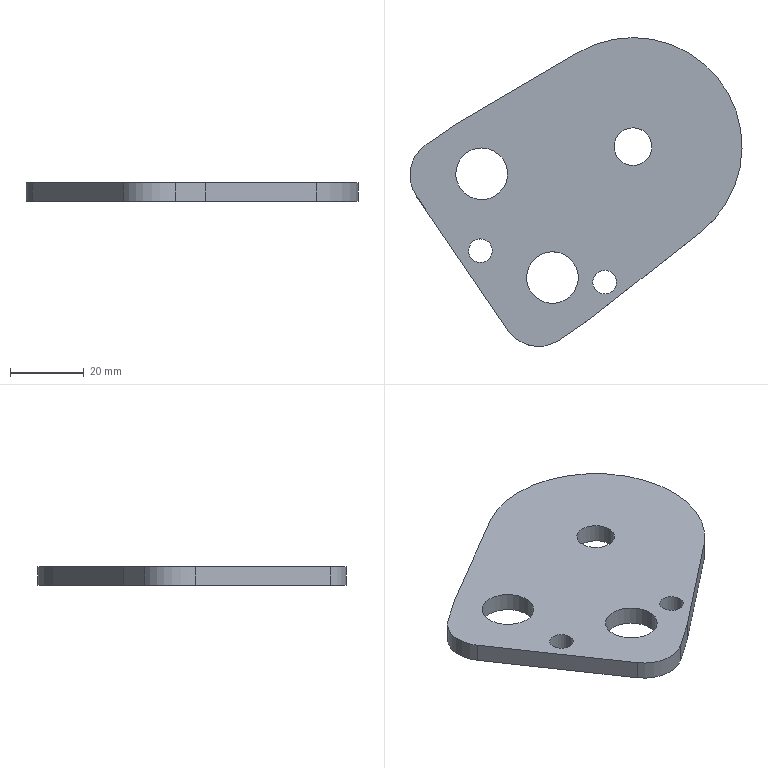Part | NX | features solid 2 | 1 solid | 15 faces | box 89.902 x 83.584 x 5 mm | volume 21833 mm3 | cylinder 8 | plane 7 | commonest cylinder face diameters 6.4 x2 14 x2 20 x2 10.2 x1 59 x1
STEP:
#1=CARTESIAN_POINT('',(-192.435,38.031,115.));
#2=VERTEX_POINT('',#1);
#3=CARTESIAN_POINT('',(-159.285,-10.613,115.));
#4=VERTEX_POINT('',#3);
#5=CARTESIAN_POINT('',(-177.504,12.589,115.));
#6=DIRECTION('',(0.,0.,-1.));
#7=DIRECTION('',(-0.8264,-0.5631,0.));
#8=AXIS2_PLACEMENT_3D('',#5,#6,#7);
#9=CIRCLE('',#8,29.5);
#10=EDGE_CURVE('',#2,#4,#9,.T.);
#11=ORIENTED_EDGE('',*,*,#10,.F.);
#12=CARTESIAN_POINT('',(-192.435,38.031,120.));
#13=VERTEX_POINT('',#12);
#14=CARTESIAN_POINT('',(-192.435,38.031,120.));
#15=DIRECTION('',(0.,0.,-1.));
#16=VECTOR('',#15,1000.);
#17=LINE('',#14,#16);
#18=EDGE_CURVE('',#13,#2,#17,.T.);
#19=ORIENTED_EDGE('',*,*,#18,.F.);
#20=CARTESIAN_POINT('',(-159.285,-10.613,120.));
#21=VERTEX_POINT('',#20);
#22=CARTESIAN_POINT('',(-177.504,12.589,120.));
#23=DIRECTION('',(0.,0.,-1.));
#24=DIRECTION('',(-0.8264,-0.5631,0.));
#25=AXIS2_PLACEMENT_3D('',#22,#23,#24);
#26=CIRCLE('',#25,29.5);
#27=EDGE_CURVE('',#13,#21,#26,.T.);
#28=ORIENTED_EDGE('',*,*,#27,.T.);
#29=CARTESIAN_POINT('',(-159.285,-10.613,120.));
#30=DIRECTION('',(0.,0.,-1.));
#31=VECTOR('',#30,1000.);
#32=LINE('',#29,#31);
#33=EDGE_CURVE('',#21,#4,#32,.T.);
#34=ORIENTED_EDGE('',*,*,#33,.T.);
#35=EDGE_LOOP('',(#11,#19,#28,#34));
#36=FACE_BOUND('',#35,.T.);
#37=CARTESIAN_POINT('',(-177.504,12.589,120.));
#38=DIRECTION('',(0.,0.,-1.));
#39=DIRECTION('',(-0.8264,-0.5631,0.));
#40=AXIS2_PLACEMENT_3D('',#37,#38,#39);
#41=CYLINDRICAL_SURFACE('',#40,29.5);
#42=ADVANCED_FACE('',(#36),#41,.T.);
#43=CARTESIAN_POINT('',(-189.232,-34.128,115.));
#44=VERTEX_POINT('',#43);
#45=CARTESIAN_POINT('',(-189.232,-34.128,115.));
#46=DIRECTION('',(0.7865,0.6176,0.));
#47=VECTOR('',#46,1000.);
#48=LINE('',#45,#47);
#49=EDGE_CURVE('',#44,#4,#48,.T.);
#50=ORIENTED_EDGE('',*,*,#49,.T.);
#51=ORIENTED_EDGE('',*,*,#33,.F.);
#52=CARTESIAN_POINT('',(-189.232,-34.128,120.));
#53=VERTEX_POINT('',#52);
#54=CARTESIAN_POINT('',(-189.232,-34.128,120.));
#55=DIRECTION('',(0.7865,0.6176,0.));
#56=VECTOR('',#55,1000.);
#57=LINE('',#54,#56);
#58=EDGE_CURVE('',#53,#21,#57,.T.);
#59=ORIENTED_EDGE('',*,*,#58,.F.);
#60=CARTESIAN_POINT('',(-189.232,-34.128,120.));
#61=DIRECTION('',(0.,0.,-1.));
#62=VECTOR('',#61,1000.);
#63=LINE('',#60,#62);
#64=EDGE_CURVE('',#53,#44,#63,.T.);
#65=ORIENTED_EDGE('',*,*,#64,.T.);
#66=EDGE_LOOP('',(#50,#51,#59,#65));
#67=FACE_BOUND('',#66,.T.);
#68=CARTESIAN_POINT('',(-189.232,-34.128,120.));
#69=DIRECTION('',(-0.6176,0.7865,0.));
#70=DIRECTION('',(0.7865,0.6176,0.));
#71=AXIS2_PLACEMENT_3D('',#68,#69,#70);
#72=PLANE('',#71);
#73=ADVANCED_FACE('',(#67),#72,.F.);
#74=CARTESIAN_POINT('',(-197.496,-39.759,120.));
#75=VERTEX_POINT('',#74);
#76=CARTESIAN_POINT('',(-189.232,-34.128,120.));
#77=DIRECTION('',(-0.8264,-0.5631,0.));
#78=VECTOR('',#77,1000.);
#79=LINE('',#76,#78);
#80=EDGE_CURVE('',#53,#75,#79,.T.);
#81=ORIENTED_EDGE('',*,*,#80,.T.);
#82=CARTESIAN_POINT('',(-197.496,-39.759,115.));
#83=VERTEX_POINT('',#82);
#84=CARTESIAN_POINT('',(-197.496,-39.759,120.));
#85=DIRECTION('',(0.,0.,-1.));
#86=VECTOR('',#85,1000.);
#87=LINE('',#84,#86);
#88=EDGE_CURVE('',#75,#83,#87,.T.);
#89=ORIENTED_EDGE('',*,*,#88,.T.);
#90=CARTESIAN_POINT('',(-189.232,-34.128,115.));
#91=DIRECTION('',(-0.8264,-0.5631,0.));
#92=VECTOR('',#91,1000.);
#93=LINE('',#90,#92);
#94=EDGE_CURVE('',#44,#83,#93,.T.);
#95=ORIENTED_EDGE('',*,*,#94,.F.);
#96=ORIENTED_EDGE('',*,*,#64,.F.);
#97=EDGE_LOOP('',(#81,#89,#95,#96));
#98=FACE_BOUND('',#97,.T.);
#99=CARTESIAN_POINT('',(-189.232,-34.128,120.));
#100=DIRECTION('',(0.5631,-0.8264,0.));
#101=DIRECTION('',(0.,0.,1.));
#102=AXIS2_PLACEMENT_3D('',#99,#100,#101);
#103=PLANE('',#102);
#104=ADVANCED_FACE('',(#98),#103,.T.);
#105=CARTESIAN_POINT('',(-211.391,-37.127,120.));
#106=VERTEX_POINT('',#105);
#107=CARTESIAN_POINT('',(-236.169,-0.7668,120.));
#108=VERTEX_POINT('',#107);
#109=CARTESIAN_POINT('',(-205.76,-45.39,120.));
#110=DIRECTION('',(-0.5631,0.8264,0.));
#111=VECTOR('',#110,1000.);
#112=LINE('',#109,#111);
#113=EDGE_CURVE('',#106,#108,#112,.T.);
#114=ORIENTED_EDGE('',*,*,#113,.T.);
#115=CARTESIAN_POINT('',(-236.169,-0.7668,115.));
#116=VERTEX_POINT('',#115);
#117=CARTESIAN_POINT('',(-236.169,-0.7668,120.));
#118=DIRECTION('',(0.,0.,-1.));
#119=VECTOR('',#118,1000.);
#120=LINE('',#117,#119);
#121=EDGE_CURVE('',#108,#116,#120,.T.);
#122=ORIENTED_EDGE('',*,*,#121,.T.);
#123=CARTESIAN_POINT('',(-211.391,-37.127,115.));
#124=VERTEX_POINT('',#123);
#125=CARTESIAN_POINT('',(-205.76,-45.39,115.));
#126=DIRECTION('',(-0.5631,0.8264,0.));
#127=VECTOR('',#126,1000.);
#128=LINE('',#125,#127);
#129=EDGE_CURVE('',#124,#116,#128,.T.);
#130=ORIENTED_EDGE('',*,*,#129,.F.);
#131=CARTESIAN_POINT('',(-211.391,-37.127,120.));
#132=DIRECTION('',(0.,0.,-1.));
#133=VECTOR('',#132,1000.);
#134=LINE('',#131,#133);
#135=EDGE_CURVE('',#124,#106,#134,.F.);
#136=ORIENTED_EDGE('',*,*,#135,.T.);
#137=EDGE_LOOP('',(#114,#122,#130,#136));
#138=FACE_BOUND('',#137,.T.);
#139=CARTESIAN_POINT('',(-205.76,-45.39,120.));
#140=DIRECTION('',(-0.8264,-0.5631,0.));
#141=DIRECTION('',(0.,0.,1.));
#142=AXIS2_PLACEMENT_3D('',#139,#140,#141);
#143=PLANE('',#142);
#144=ADVANCED_FACE('',(#138),#143,.T.);
#145=CARTESIAN_POINT('',(-233.537,13.128,115.));
#146=VERTEX_POINT('',#145);
#147=CARTESIAN_POINT('',(-225.273,18.76,115.));
#148=VERTEX_POINT('',#147);
#149=CARTESIAN_POINT('',(-241.8,7.497,115.));
#150=DIRECTION('',(0.8264,0.5631,0.));
#151=VECTOR('',#150,1000.);
#152=LINE('',#149,#151);
#153=EDGE_CURVE('',#146,#148,#152,.T.);
#154=ORIENTED_EDGE('',*,*,#153,.F.);
#155=CARTESIAN_POINT('',(-233.537,13.128,120.));
#156=VERTEX_POINT('',#155);
#157=CARTESIAN_POINT('',(-233.537,13.128,120.));
#158=DIRECTION('',(0.,0.,-1.));
#159=VECTOR('',#158,1000.);
#160=LINE('',#157,#159);
#161=EDGE_CURVE('',#146,#156,#160,.F.);
#162=ORIENTED_EDGE('',*,*,#161,.T.);
#163=CARTESIAN_POINT('',(-225.273,18.76,120.));
#164=VERTEX_POINT('',#163);
#165=CARTESIAN_POINT('',(-241.8,7.497,120.));
#166=DIRECTION('',(0.8264,0.5631,0.));
#167=VECTOR('',#166,1000.);
#168=LINE('',#165,#167);
#169=EDGE_CURVE('',#156,#164,#168,.T.);
#170=ORIENTED_EDGE('',*,*,#169,.T.);
#171=CARTESIAN_POINT('',(-225.273,18.76,120.));
#172=DIRECTION('',(0.,0.,-1.));
#173=VECTOR('',#172,1000.);
#174=LINE('',#171,#173);
#175=EDGE_CURVE('',#164,#148,#174,.T.);
#176=ORIENTED_EDGE('',*,*,#175,.T.);
#177=EDGE_LOOP('',(#154,#162,#170,#176));
#178=FACE_BOUND('',#177,.T.);
#179=CARTESIAN_POINT('',(-241.8,7.497,120.));
#180=DIRECTION('',(-0.5631,0.8264,0.));
#181=DIRECTION('',(0.,0.,-1.));
#182=AXIS2_PLACEMENT_3D('',#179,#180,#181);
#183=PLANE('',#182);
#184=ADVANCED_FACE('',(#178),#183,.T.);
#185=CARTESIAN_POINT('',(-181.718,9.717,120.));
#186=VERTEX_POINT('',#185);
#187=CARTESIAN_POINT('',(-177.504,12.589,120.));
#188=DIRECTION('',(0.,0.,-1.));
#189=DIRECTION('',(-0.8264,-0.5631,0.));
#190=AXIS2_PLACEMENT_3D('',#187,#188,#189);
#191=CIRCLE('',#190,5.1);
#192=EDGE_CURVE('',#186,#186,#191,.T.);
#193=ORIENTED_EDGE('',*,*,#192,.F.);
#194=EDGE_LOOP('',(#193));
#195=FACE_BOUND('',#194,.T.);
#196=CARTESIAN_POINT('',(-181.718,9.717,115.));
#197=VERTEX_POINT('',#196);
#198=CARTESIAN_POINT('',(-177.504,12.589,115.));
#199=DIRECTION('',(0.,0.,-1.));
#200=DIRECTION('',(-0.8264,-0.5631,0.));
#201=AXIS2_PLACEMENT_3D('',#198,#199,#200);
#202=CIRCLE('',#201,5.1);
#203=EDGE_CURVE('',#197,#197,#202,.T.);
#204=ORIENTED_EDGE('',*,*,#203,.T.);
#205=EDGE_LOOP('',(#204));
#206=FACE_BOUND('',#205,.T.);
#207=CARTESIAN_POINT('',(-177.504,12.589,120.));
#208=DIRECTION('',(0.,0.,-1.));
#209=DIRECTION('',(-0.8264,-0.5631,0.));
#210=AXIS2_PLACEMENT_3D('',#207,#208,#209);
#211=CYLINDRICAL_SURFACE('',#210,5.1);
#212=ADVANCED_FACE('',(#195,#206),#211,.F.);
#213=CARTESIAN_POINT('',(-205.117,-26.8,120.));
#214=VERTEX_POINT('',#213);
#215=CARTESIAN_POINT('',(-199.332,-22.858,120.));
#216=DIRECTION('',(0.,0.,-1.));
#217=DIRECTION('',(-0.8264,-0.5631,0.));
#218=AXIS2_PLACEMENT_3D('',#215,#216,#217);
#219=CIRCLE('',#218,7.);
#220=EDGE_CURVE('',#214,#214,#219,.T.);
#221=ORIENTED_EDGE('',*,*,#220,.F.);
#222=EDGE_LOOP('',(#221));
#223=FACE_BOUND('',#222,.T.);
#224=CARTESIAN_POINT('',(-205.117,-26.8,115.));
#225=VERTEX_POINT('',#224);
#226=CARTESIAN_POINT('',(-199.332,-22.858,115.));
#227=DIRECTION('',(0.,0.,-1.));
#228=DIRECTION('',(-0.8264,-0.5631,0.));
#229=AXIS2_PLACEMENT_3D('',#226,#227,#228);
#230=CIRCLE('',#229,7.);
#231=EDGE_CURVE('',#225,#225,#230,.T.);
#232=ORIENTED_EDGE('',*,*,#231,.T.);
#233=EDGE_LOOP('',(#232));
#234=FACE_BOUND('',#233,.T.);
#235=CARTESIAN_POINT('',(-199.332,-22.858,120.));
#236=DIRECTION('',(0.,0.,-1.));
#237=DIRECTION('',(-0.8264,-0.5631,0.));
#238=AXIS2_PLACEMENT_3D('',#235,#236,#237);
#239=CYLINDRICAL_SURFACE('',#238,7.);
#240=ADVANCED_FACE('',(#223,#234),#239,.F.);
#241=CARTESIAN_POINT('',(-224.263,1.296,120.));
#242=VERTEX_POINT('',#241);
#243=CARTESIAN_POINT('',(-218.479,5.238,120.));
#244=DIRECTION('',(0.,0.,-1.));
#245=DIRECTION('',(-0.8264,-0.5631,0.));
#246=AXIS2_PLACEMENT_3D('',#243,#244,#245);
#247=CIRCLE('',#246,7.);
#248=EDGE_CURVE('',#242,#242,#247,.T.);
#249=ORIENTED_EDGE('',*,*,#248,.F.);
#250=EDGE_LOOP('',(#249));
#251=FACE_BOUND('',#250,.T.);
#252=CARTESIAN_POINT('',(-224.263,1.296,115.));
#253=VERTEX_POINT('',#252);
#254=CARTESIAN_POINT('',(-218.479,5.238,115.));
#255=DIRECTION('',(0.,0.,-1.));
#256=DIRECTION('',(-0.8264,-0.5631,0.));
#257=AXIS2_PLACEMENT_3D('',#254,#255,#256);
#258=CIRCLE('',#257,7.);
#259=EDGE_CURVE('',#253,#253,#258,.T.);
#260=ORIENTED_EDGE('',*,*,#259,.T.);
#261=EDGE_LOOP('',(#260));
#262=FACE_BOUND('',#261,.T.);
#263=CARTESIAN_POINT('',(-218.479,5.238,120.));
#264=DIRECTION('',(0.,0.,-1.));
#265=DIRECTION('',(-0.8264,-0.5631,0.));
#266=AXIS2_PLACEMENT_3D('',#263,#264,#265);
#267=CYLINDRICAL_SURFACE('',#266,7.);
#268=ADVANCED_FACE('',(#251,#262),#267,.F.);
#269=CARTESIAN_POINT('',(-221.466,-17.37,120.));
#270=VERTEX_POINT('',#269);
#271=CARTESIAN_POINT('',(-218.822,-15.568,120.));
#272=DIRECTION('',(0.,0.,-1.));
#273=DIRECTION('',(-0.8264,-0.5631,0.));
#274=AXIS2_PLACEMENT_3D('',#271,#272,#273);
#275=CIRCLE('',#274,3.2);
#276=EDGE_CURVE('',#270,#270,#275,.T.);
#277=ORIENTED_EDGE('',*,*,#276,.F.);
#278=EDGE_LOOP('',(#277));
#279=FACE_BOUND('',#278,.T.);
#280=CARTESIAN_POINT('',(-221.466,-17.37,115.));
#281=VERTEX_POINT('',#280);
#282=CARTESIAN_POINT('',(-218.822,-15.568,115.));
#283=DIRECTION('',(0.,0.,-1.));
#284=DIRECTION('',(-0.8264,-0.5631,0.));
#285=AXIS2_PLACEMENT_3D('',#282,#283,#284);
#286=CIRCLE('',#285,3.2);
#287=EDGE_CURVE('',#281,#281,#286,.T.);
#288=ORIENTED_EDGE('',*,*,#287,.T.);
#289=EDGE_LOOP('',(#288));
#290=FACE_BOUND('',#289,.T.);
#291=CARTESIAN_POINT('',(-218.822,-15.568,120.));
#292=DIRECTION('',(0.,0.,-1.));
#293=DIRECTION('',(-0.8264,-0.5631,0.));
#294=AXIS2_PLACEMENT_3D('',#291,#292,#293);
#295=CYLINDRICAL_SURFACE('',#294,3.2);
#296=ADVANCED_FACE('',(#279,#290),#295,.F.);
#297=CARTESIAN_POINT('',(-187.818,-25.903,120.));
#298=VERTEX_POINT('',#297);
#299=CARTESIAN_POINT('',(-185.174,-24.101,120.));
#300=DIRECTION('',(0.,0.,-1.));
#301=DIRECTION('',(-0.8264,-0.5631,0.));
#302=AXIS2_PLACEMENT_3D('',#299,#300,#301);
#303=CIRCLE('',#302,3.2);
#304=EDGE_CURVE('',#298,#298,#303,.T.);
#305=ORIENTED_EDGE('',*,*,#304,.F.);
#306=EDGE_LOOP('',(#305));
#307=FACE_BOUND('',#306,.T.);
#308=CARTESIAN_POINT('',(-187.818,-25.903,115.));
#309=VERTEX_POINT('',#308);
#310=CARTESIAN_POINT('',(-185.174,-24.101,115.));
#311=DIRECTION('',(0.,0.,-1.));
#312=DIRECTION('',(-0.8264,-0.5631,0.));
#313=AXIS2_PLACEMENT_3D('',#310,#311,#312);
#314=CIRCLE('',#313,3.2);
#315=EDGE_CURVE('',#309,#309,#314,.T.);
#316=ORIENTED_EDGE('',*,*,#315,.T.);
#317=EDGE_LOOP('',(#316));
#318=FACE_BOUND('',#317,.T.);
#319=CARTESIAN_POINT('',(-185.174,-24.101,120.));
#320=DIRECTION('',(0.,0.,-1.));
#321=DIRECTION('',(-0.8264,-0.5631,0.));
#322=AXIS2_PLACEMENT_3D('',#319,#320,#321);
#323=CYLINDRICAL_SURFACE('',#322,3.2);
#324=ADVANCED_FACE('',(#307,#318),#323,.F.);
#325=CARTESIAN_POINT('',(-225.273,18.76,115.));
#326=DIRECTION('',(0.8624,0.5061,0.));
#327=VECTOR('',#326,1000.);
#328=LINE('',#325,#327);
#329=EDGE_CURVE('',#148,#2,#328,.T.);
#330=ORIENTED_EDGE('',*,*,#329,.F.);
#331=ORIENTED_EDGE('',*,*,#175,.F.);
#332=CARTESIAN_POINT('',(-225.273,18.76,120.));
#333=DIRECTION('',(0.8624,0.5061,0.));
#334=VECTOR('',#333,1000.);
#335=LINE('',#332,#334);
#336=EDGE_CURVE('',#164,#13,#335,.T.);
#337=ORIENTED_EDGE('',*,*,#336,.T.);
#338=ORIENTED_EDGE('',*,*,#18,.T.);
#339=EDGE_LOOP('',(#330,#331,#337,#338));
#340=FACE_BOUND('',#339,.T.);
#341=CARTESIAN_POINT('',(-225.273,18.76,120.));
#342=DIRECTION('',(-0.5061,0.8624,0.));
#343=DIRECTION('',(0.8624,0.5061,0.));
#344=AXIS2_PLACEMENT_3D('',#341,#342,#343);
#345=PLANE('',#344);
#346=ADVANCED_FACE('',(#340),#345,.T.);
#347=ORIENTED_EDGE('',*,*,#304,.T.);
#348=EDGE_LOOP('',(#347));
#349=FACE_BOUND('',#348,.T.);
#350=ORIENTED_EDGE('',*,*,#276,.T.);
#351=EDGE_LOOP('',(#350));
#352=FACE_BOUND('',#351,.T.);
#353=ORIENTED_EDGE('',*,*,#248,.T.);
#354=EDGE_LOOP('',(#353));
#355=FACE_BOUND('',#354,.T.);
#356=ORIENTED_EDGE('',*,*,#220,.T.);
#357=EDGE_LOOP('',(#356));
#358=FACE_BOUND('',#357,.T.);
#359=ORIENTED_EDGE('',*,*,#192,.T.);
#360=EDGE_LOOP('',(#359));
#361=FACE_BOUND('',#360,.T.);
#362=ORIENTED_EDGE('',*,*,#169,.F.);
#363=CARTESIAN_POINT('',(-227.905,4.865,120.));
#364=DIRECTION('',(0.,0.,-1.));
#365=DIRECTION('',(-0.8264,-0.5631,0.));
#366=AXIS2_PLACEMENT_3D('',#363,#364,#365);
#367=CIRCLE('',#366,10.);
#368=EDGE_CURVE('',#156,#108,#367,.F.);
#369=ORIENTED_EDGE('',*,*,#368,.T.);
#370=ORIENTED_EDGE('',*,*,#113,.F.);
#371=CARTESIAN_POINT('',(-203.127,-31.495,120.));
#372=DIRECTION('',(0.,0.,-1.));
#373=DIRECTION('',(-0.8264,-0.5631,0.));
#374=AXIS2_PLACEMENT_3D('',#371,#372,#373);
#375=CIRCLE('',#374,10.);
#376=EDGE_CURVE('',#106,#75,#375,.F.);
#377=ORIENTED_EDGE('',*,*,#376,.T.);
#378=ORIENTED_EDGE('',*,*,#80,.F.);
#379=ORIENTED_EDGE('',*,*,#58,.T.);
#380=ORIENTED_EDGE('',*,*,#27,.F.);
#381=ORIENTED_EDGE('',*,*,#336,.F.);
#382=EDGE_LOOP('',(#362,#369,#370,#377,#378,#379,#380,#381));
#383=FACE_BOUND('',#382,.T.);
#384=CARTESIAN_POINT('',(-177.504,12.589,120.));
#385=DIRECTION('',(0.,0.,-1.));
#386=DIRECTION('',(-0.8264,-0.5631,0.));
#387=AXIS2_PLACEMENT_3D('',#384,#385,#386);
#388=PLANE('',#387);
#389=ADVANCED_FACE('',(#349,#352,#355,#358,#361,#383),#388,.F.);
#390=ORIENTED_EDGE('',*,*,#315,.F.);
#391=EDGE_LOOP('',(#390));
#392=FACE_BOUND('',#391,.T.);
#393=ORIENTED_EDGE('',*,*,#287,.F.);
#394=EDGE_LOOP('',(#393));
#395=FACE_BOUND('',#394,.T.);
#396=ORIENTED_EDGE('',*,*,#259,.F.);
#397=EDGE_LOOP('',(#396));
#398=FACE_BOUND('',#397,.T.);
#399=ORIENTED_EDGE('',*,*,#231,.F.);
#400=EDGE_LOOP('',(#399));
#401=FACE_BOUND('',#400,.T.);
#402=ORIENTED_EDGE('',*,*,#203,.F.);
#403=EDGE_LOOP('',(#402));
#404=FACE_BOUND('',#403,.T.);
#405=ORIENTED_EDGE('',*,*,#129,.T.);
#406=CARTESIAN_POINT('',(-227.905,4.865,115.));
#407=DIRECTION('',(0.,0.,-1.));
#408=DIRECTION('',(-0.8264,-0.5631,0.));
#409=AXIS2_PLACEMENT_3D('',#406,#407,#408);
#410=CIRCLE('',#409,10.);
#411=EDGE_CURVE('',#116,#146,#410,.T.);
#412=ORIENTED_EDGE('',*,*,#411,.T.);
#413=ORIENTED_EDGE('',*,*,#153,.T.);
#414=ORIENTED_EDGE('',*,*,#329,.T.);
#415=ORIENTED_EDGE('',*,*,#10,.T.);
#416=ORIENTED_EDGE('',*,*,#49,.F.);
#417=ORIENTED_EDGE('',*,*,#94,.T.);
#418=CARTESIAN_POINT('',(-203.127,-31.495,115.));
#419=DIRECTION('',(0.,0.,-1.));
#420=DIRECTION('',(-0.8264,-0.5631,0.));
#421=AXIS2_PLACEMENT_3D('',#418,#419,#420);
#422=CIRCLE('',#421,10.);
#423=EDGE_CURVE('',#83,#124,#422,.T.);
#424=ORIENTED_EDGE('',*,*,#423,.T.);
#425=EDGE_LOOP('',(#405,#412,#413,#414,#415,#416,#417,#424));
#426=FACE_BOUND('',#425,.T.);
#427=CARTESIAN_POINT('',(-177.504,12.589,115.));
#428=DIRECTION('',(0.,0.,-1.));
#429=DIRECTION('',(-0.8264,-0.5631,0.));
#430=AXIS2_PLACEMENT_3D('',#427,#428,#429);
#431=PLANE('',#430);
#432=ADVANCED_FACE('',(#392,#395,#398,#401,#404,#426),#431,.T.);
#433=ORIENTED_EDGE('',*,*,#368,.F.);
#434=ORIENTED_EDGE('',*,*,#161,.F.);
#435=ORIENTED_EDGE('',*,*,#411,.F.);
#436=ORIENTED_EDGE('',*,*,#121,.F.);
#437=EDGE_LOOP('',(#433,#434,#435,#436));
#438=FACE_BOUND('',#437,.T.);
#439=CARTESIAN_POINT('',(-227.905,4.865,120.));
#440=DIRECTION('',(0.,0.,-1.));
#441=DIRECTION('',(-0.8264,-0.5631,0.));
#442=AXIS2_PLACEMENT_3D('',#439,#440,#441);
#443=CYLINDRICAL_SURFACE('',#442,10.);
#444=ADVANCED_FACE('',(#438),#443,.T.);
#445=ORIENTED_EDGE('',*,*,#376,.F.);
#446=ORIENTED_EDGE('',*,*,#135,.F.);
#447=ORIENTED_EDGE('',*,*,#423,.F.);
#448=ORIENTED_EDGE('',*,*,#88,.F.);
#449=EDGE_LOOP('',(#445,#446,#447,#448));
#450=FACE_BOUND('',#449,.T.);
#451=CARTESIAN_POINT('',(-203.127,-31.495,120.));
#452=DIRECTION('',(0.,0.,-1.));
#453=DIRECTION('',(-0.8264,-0.5631,0.));
#454=AXIS2_PLACEMENT_3D('',#451,#452,#453);
#455=CYLINDRICAL_SURFACE('',#454,10.);
#456=ADVANCED_FACE('',(#450),#455,.T.);
#457=CLOSED_SHELL('',(#42,#73,#104,#144,#184,#212,#240,#268,#296,#324,#346,#389,#432,#444,#456));
#458=MANIFOLD_SOLID_BREP('',#457);
#459=(LENGTH_UNIT()NAMED_UNIT(*)SI_UNIT(.MILLI.,.METRE.));
#460=UNCERTAINTY_MEASURE_WITH_UNIT(LENGTH_MEASURE(0.00001),#459,'','');
#461=(NAMED_UNIT(*)PLANE_ANGLE_UNIT()SI_UNIT($,.RADIAN.));
#462=(NAMED_UNIT(*)SI_UNIT($,.STERADIAN.)SOLID_ANGLE_UNIT());
#463=(GEOMETRIC_REPRESENTATION_CONTEXT(3)GLOBAL_UNCERTAINTY_ASSIGNED_CONTEXT((#460))GLOBAL_UNIT_ASSIGNED_CONTEXT((#459,#461,#462))REPRESENTATION_CONTEXT('',''));
#464=ADVANCED_BREP_SHAPE_REPRESENTATION('',(#458),#463);